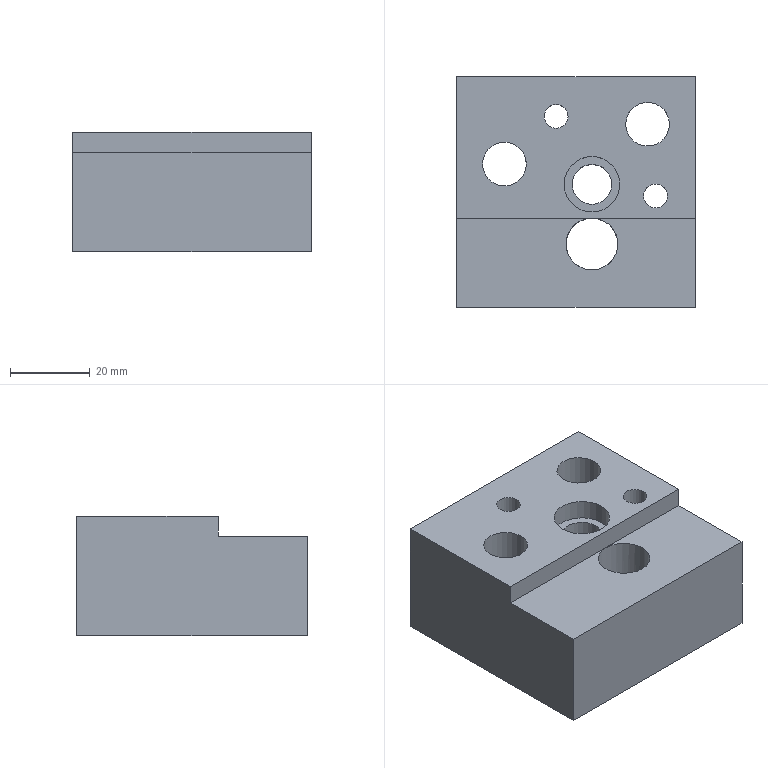Part | NX | features solid 2 | 1 solid | 20 faces | box 60 x 58 x 30 mm | volume 80735 mm3 | plane 11 | cylinder 9 | commonest cylinder face diameters 6 x2 11 x2 17.5 x2 10 x1 13 x1 14 x1
STEP:
#1=CARTESIAN_POINT('',(-695.999,-287.091,74.));
#2=VERTEX_POINT('',#1);
#3=CARTESIAN_POINT('',(-690.999,-287.091,74.));
#4=DIRECTION('',(0.,0.,-1.));
#5=DIRECTION('',(-1.,0.,0.));
#6=AXIS2_PLACEMENT_3D('',#3,#4,#5);
#7=CIRCLE('',#6,5.);
#8=EDGE_CURVE('',#2,#2,#7,.F.);
#9=ORIENTED_EDGE('',*,*,#8,.T.);
#10=EDGE_LOOP('',(#9));
#11=FACE_BOUND('',#10,.T.);
#12=CARTESIAN_POINT('',(-725.,-260.,74.));
#13=VERTEX_POINT('',#12);
#14=CARTESIAN_POINT('',(-665.,-260.,74.));
#15=VERTEX_POINT('',#14);
#16=CARTESIAN_POINT('',(-695.663,-260.,74.));
#17=DIRECTION('',(1.,0.,0.));
#18=VECTOR('',#17,1000.);
#19=LINE('',#16,#18);
#20=EDGE_CURVE('',#13,#15,#19,.T.);
#21=ORIENTED_EDGE('',*,*,#20,.T.);
#22=CARTESIAN_POINT('',(-665.,-318.,74.));
#23=VERTEX_POINT('',#22);
#24=CARTESIAN_POINT('',(-665.,-290.591,74.));
#25=DIRECTION('',(0.,-1.,0.));
#26=VECTOR('',#25,1000.);
#27=LINE('',#24,#26);
#28=EDGE_CURVE('',#15,#23,#27,.T.);
#29=ORIENTED_EDGE('',*,*,#28,.T.);
#30=CARTESIAN_POINT('',(-725.,-318.,74.));
#31=VERTEX_POINT('',#30);
#32=CARTESIAN_POINT('',(-695.663,-318.,74.));
#33=DIRECTION('',(1.,0.,0.));
#34=VECTOR('',#33,1000.);
#35=LINE('',#32,#34);
#36=EDGE_CURVE('',#31,#23,#35,.T.);
#37=ORIENTED_EDGE('',*,*,#36,.F.);
#38=CARTESIAN_POINT('',(-725.,-290.591,74.));
#39=DIRECTION('',(0.,-1.,0.));
#40=VECTOR('',#39,1000.);
#41=LINE('',#38,#40);
#42=EDGE_CURVE('',#13,#31,#41,.T.);
#43=ORIENTED_EDGE('',*,*,#42,.F.);
#44=EDGE_LOOP('',(#21,#29,#37,#43));
#45=FACE_BOUND('',#44,.T.);
#46=CARTESIAN_POINT('',(-668.25,-272.,74.));
#47=VERTEX_POINT('',#46);
#48=CARTESIAN_POINT('',(-677.,-272.,74.));
#49=DIRECTION('',(0.,0.,1.));
#50=DIRECTION('',(1.,0.,0.));
#51=AXIS2_PLACEMENT_3D('',#48,#49,#50);
#52=CIRCLE('',#51,8.75);
#53=EDGE_CURVE('',#47,#47,#52,.T.);
#54=ORIENTED_EDGE('',*,*,#53,.T.);
#55=EDGE_LOOP('',(#54));
#56=FACE_BOUND('',#55,.T.);
#57=CARTESIAN_POINT('',(-704.25,-282.,74.));
#58=VERTEX_POINT('',#57);
#59=CARTESIAN_POINT('',(-713.,-282.,74.));
#60=DIRECTION('',(0.,0.,1.));
#61=DIRECTION('',(1.,0.,0.));
#62=AXIS2_PLACEMENT_3D('',#59,#60,#61);
#63=CIRCLE('',#62,8.75);
#64=EDGE_CURVE('',#58,#58,#63,.T.);
#65=ORIENTED_EDGE('',*,*,#64,.T.);
#66=EDGE_LOOP('',(#65));
#67=FACE_BOUND('',#66,.T.);
#68=CARTESIAN_POINT('',(-697.,-270.,74.));
#69=VERTEX_POINT('',#68);
#70=CARTESIAN_POINT('',(-700.,-270.,74.));
#71=DIRECTION('',(0.,0.,1.));
#72=DIRECTION('',(1.,0.,0.));
#73=AXIS2_PLACEMENT_3D('',#70,#71,#72);
#74=CIRCLE('',#73,3.);
#75=EDGE_CURVE('',#69,#69,#74,.T.);
#76=ORIENTED_EDGE('',*,*,#75,.T.);
#77=EDGE_LOOP('',(#76));
#78=FACE_BOUND('',#77,.T.);
#79=CARTESIAN_POINT('',(-672.,-290.,74.));
#80=VERTEX_POINT('',#79);
#81=CARTESIAN_POINT('',(-675.,-290.,74.));
#82=DIRECTION('',(0.,0.,1.));
#83=DIRECTION('',(1.,0.,0.));
#84=AXIS2_PLACEMENT_3D('',#81,#82,#83);
#85=CIRCLE('',#84,3.);
#86=EDGE_CURVE('',#80,#80,#85,.T.);
#87=ORIENTED_EDGE('',*,*,#86,.T.);
#88=EDGE_LOOP('',(#87));
#89=FACE_BOUND('',#88,.T.);
#90=CARTESIAN_POINT('',(-684.499,-302.091,74.));
#91=VERTEX_POINT('',#90);
#92=CARTESIAN_POINT('',(-690.999,-302.091,74.));
#93=DIRECTION('',(0.,0.,1.));
#94=DIRECTION('',(1.,0.,0.));
#95=AXIS2_PLACEMENT_3D('',#92,#93,#94);
#96=CIRCLE('',#95,6.5);
#97=EDGE_CURVE('',#91,#91,#96,.F.);
#98=ORIENTED_EDGE('',*,*,#97,.F.);
#99=EDGE_LOOP('',(#98));
#100=FACE_BOUND('',#99,.T.);
#101=CARTESIAN_POINT('',(-695.663,-290.591,74.));
#102=DIRECTION('',(0.,0.,-1.));
#103=DIRECTION('',(-1.,0.,0.));
#104=AXIS2_PLACEMENT_3D('',#101,#102,#103);
#105=PLANE('',#104);
#106=ADVANCED_FACE('',(#11,#45,#56,#67,#78,#89,#100),#105,.T.);
#107=CARTESIAN_POINT('',(-665.,-295.591,99.));
#108=VERTEX_POINT('',#107);
#109=CARTESIAN_POINT('',(-665.,-295.591,104.));
#110=VERTEX_POINT('',#109);
#111=CARTESIAN_POINT('',(-665.,-295.591,107.));
#112=DIRECTION('',(0.,0.,1.));
#113=VECTOR('',#112,1000.);
#114=LINE('',#111,#113);
#115=EDGE_CURVE('',#108,#110,#114,.T.);
#116=ORIENTED_EDGE('',*,*,#115,.F.);
#117=CARTESIAN_POINT('',(-665.,-318.,99.));
#118=VERTEX_POINT('',#117);
#119=CARTESIAN_POINT('',(-665.,-302.091,99.));
#120=DIRECTION('',(0.,1.,0.));
#121=VECTOR('',#120,1000.);
#122=LINE('',#119,#121);
#123=EDGE_CURVE('',#108,#118,#122,.F.);
#124=ORIENTED_EDGE('',*,*,#123,.T.);
#125=CARTESIAN_POINT('',(-665.,-318.,0.));
#126=DIRECTION('',(0.,0.,-1.));
#127=VECTOR('',#126,1000.);
#128=LINE('',#125,#127);
#129=EDGE_CURVE('',#118,#23,#128,.T.);
#130=ORIENTED_EDGE('',*,*,#129,.T.);
#131=ORIENTED_EDGE('',*,*,#28,.F.);
#132=CARTESIAN_POINT('',(-665.,-260.,104.));
#133=VERTEX_POINT('',#132);
#134=CARTESIAN_POINT('',(-665.,-260.,0.));
#135=DIRECTION('',(0.,0.,-1.));
#136=VECTOR('',#135,1000.);
#137=LINE('',#134,#136);
#138=EDGE_CURVE('',#133,#15,#137,.T.);
#139=ORIENTED_EDGE('',*,*,#138,.F.);
#140=CARTESIAN_POINT('',(-665.,-302.091,104.));
#141=DIRECTION('',(0.,1.,0.));
#142=VECTOR('',#141,1000.);
#143=LINE('',#140,#142);
#144=EDGE_CURVE('',#133,#110,#143,.F.);
#145=ORIENTED_EDGE('',*,*,#144,.T.);
#146=EDGE_LOOP('',(#116,#124,#130,#131,#139,#145));
#147=FACE_BOUND('',#146,.T.);
#148=CARTESIAN_POINT('',(-665.,0.,0.));
#149=DIRECTION('',(1.,0.,0.));
#150=DIRECTION('',(0.,0.,-1.));
#151=AXIS2_PLACEMENT_3D('',#148,#149,#150);
#152=PLANE('',#151);
#153=ADVANCED_FACE('',(#147),#152,.T.);
#154=CARTESIAN_POINT('',(-725.,-260.,104.));
#155=VERTEX_POINT('',#154);
#156=CARTESIAN_POINT('',(-725.,-260.,0.));
#157=DIRECTION('',(0.,0.,-1.));
#158=VECTOR('',#157,1000.);
#159=LINE('',#156,#158);
#160=EDGE_CURVE('',#155,#13,#159,.T.);
#161=ORIENTED_EDGE('',*,*,#160,.T.);
#162=ORIENTED_EDGE('',*,*,#42,.T.);
#163=CARTESIAN_POINT('',(-725.,-318.,99.));
#164=VERTEX_POINT('',#163);
#165=CARTESIAN_POINT('',(-725.,-318.,0.));
#166=DIRECTION('',(0.,0.,-1.));
#167=VECTOR('',#166,1000.);
#168=LINE('',#165,#167);
#169=EDGE_CURVE('',#164,#31,#168,.T.);
#170=ORIENTED_EDGE('',*,*,#169,.F.);
#171=CARTESIAN_POINT('',(-725.,-295.591,99.));
#172=VERTEX_POINT('',#171);
#173=CARTESIAN_POINT('',(-725.,-302.091,99.));
#174=DIRECTION('',(0.,1.,0.));
#175=VECTOR('',#174,1000.);
#176=LINE('',#173,#175);
#177=EDGE_CURVE('',#172,#164,#176,.F.);
#178=ORIENTED_EDGE('',*,*,#177,.F.);
#179=CARTESIAN_POINT('',(-725.,-295.591,104.));
#180=VERTEX_POINT('',#179);
#181=CARTESIAN_POINT('',(-725.,-295.591,107.));
#182=DIRECTION('',(0.,0.,1.));
#183=VECTOR('',#182,1000.);
#184=LINE('',#181,#183);
#185=EDGE_CURVE('',#172,#180,#184,.T.);
#186=ORIENTED_EDGE('',*,*,#185,.T.);
#187=CARTESIAN_POINT('',(-725.,-302.091,104.));
#188=DIRECTION('',(0.,1.,0.));
#189=VECTOR('',#188,1000.);
#190=LINE('',#187,#189);
#191=EDGE_CURVE('',#155,#180,#190,.F.);
#192=ORIENTED_EDGE('',*,*,#191,.F.);
#193=EDGE_LOOP('',(#161,#162,#170,#178,#186,#192));
#194=FACE_BOUND('',#193,.T.);
#195=CARTESIAN_POINT('',(-725.,0.,0.));
#196=DIRECTION('',(1.,0.,0.));
#197=DIRECTION('',(0.,0.,-1.));
#198=AXIS2_PLACEMENT_3D('',#195,#196,#197);
#199=PLANE('',#198);
#200=ADVANCED_FACE('',(#194),#199,.F.);
#201=CARTESIAN_POINT('',(-672.,-290.,104.));
#202=VERTEX_POINT('',#201);
#203=CARTESIAN_POINT('',(-675.,-290.,104.));
#204=DIRECTION('',(0.,0.,1.));
#205=DIRECTION('',(1.,0.,0.));
#206=AXIS2_PLACEMENT_3D('',#203,#204,#205);
#207=CIRCLE('',#206,3.);
#208=EDGE_CURVE('',#202,#202,#207,.F.);
#209=ORIENTED_EDGE('',*,*,#208,.T.);
#210=EDGE_LOOP('',(#209));
#211=FACE_BOUND('',#210,.T.);
#212=CARTESIAN_POINT('',(-697.,-270.,104.));
#213=VERTEX_POINT('',#212);
#214=CARTESIAN_POINT('',(-700.,-270.,104.));
#215=DIRECTION('',(0.,0.,1.));
#216=DIRECTION('',(1.,0.,0.));
#217=AXIS2_PLACEMENT_3D('',#214,#215,#216);
#218=CIRCLE('',#217,3.);
#219=EDGE_CURVE('',#213,#213,#218,.F.);
#220=ORIENTED_EDGE('',*,*,#219,.T.);
#221=EDGE_LOOP('',(#220));
#222=FACE_BOUND('',#221,.T.);
#223=CARTESIAN_POINT('',(-707.5,-282.,104.));
#224=VERTEX_POINT('',#223);
#225=CARTESIAN_POINT('',(-713.,-282.,104.));
#226=DIRECTION('',(0.,0.,1.));
#227=DIRECTION('',(1.,0.,0.));
#228=AXIS2_PLACEMENT_3D('',#225,#226,#227);
#229=CIRCLE('',#228,5.5);
#230=EDGE_CURVE('',#224,#224,#229,.F.);
#231=ORIENTED_EDGE('',*,*,#230,.T.);
#232=EDGE_LOOP('',(#231));
#233=FACE_BOUND('',#232,.T.);
#234=CARTESIAN_POINT('',(-671.5,-272.,104.));
#235=VERTEX_POINT('',#234);
#236=CARTESIAN_POINT('',(-677.,-272.,104.));
#237=DIRECTION('',(0.,0.,1.));
#238=DIRECTION('',(1.,0.,0.));
#239=AXIS2_PLACEMENT_3D('',#236,#237,#238);
#240=CIRCLE('',#239,5.5);
#241=EDGE_CURVE('',#235,#235,#240,.F.);
#242=ORIENTED_EDGE('',*,*,#241,.T.);
#243=EDGE_LOOP('',(#242));
#244=FACE_BOUND('',#243,.T.);
#245=CARTESIAN_POINT('',(-697.999,-287.091,104.));
#246=VERTEX_POINT('',#245);
#247=CARTESIAN_POINT('',(-690.999,-287.091,104.));
#248=DIRECTION('',(0.,0.,-1.));
#249=DIRECTION('',(-1.,0.,0.));
#250=AXIS2_PLACEMENT_3D('',#247,#248,#249);
#251=CIRCLE('',#250,7.);
#252=EDGE_CURVE('',#246,#246,#251,.F.);
#253=ORIENTED_EDGE('',*,*,#252,.F.);
#254=EDGE_LOOP('',(#253));
#255=FACE_BOUND('',#254,.T.);
#256=ORIENTED_EDGE('',*,*,#144,.F.);
#257=CARTESIAN_POINT('',(-690.999,-260.,104.));
#258=DIRECTION('',(-1.,0.,0.));
#259=VECTOR('',#258,1000.);
#260=LINE('',#257,#259);
#261=EDGE_CURVE('',#155,#133,#260,.F.);
#262=ORIENTED_EDGE('',*,*,#261,.F.);
#263=ORIENTED_EDGE('',*,*,#191,.T.);
#264=CARTESIAN_POINT('',(-686.336,-295.591,104.));
#265=DIRECTION('',(-1.,0.,0.));
#266=VECTOR('',#265,1000.);
#267=LINE('',#264,#266);
#268=EDGE_CURVE('',#180,#110,#267,.F.);
#269=ORIENTED_EDGE('',*,*,#268,.T.);
#270=EDGE_LOOP('',(#256,#262,#263,#269));
#271=FACE_BOUND('',#270,.T.);
#272=CARTESIAN_POINT('',(-690.999,-302.091,104.));
#273=DIRECTION('',(0.,0.,1.));
#274=DIRECTION('',(0.,-1.,0.));
#275=AXIS2_PLACEMENT_3D('',#272,#273,#274);
#276=PLANE('',#275);
#277=ADVANCED_FACE('',(#211,#222,#233,#244,#255,#271),#276,.T.);
#278=ORIENTED_EDGE('',*,*,#261,.T.);
#279=ORIENTED_EDGE('',*,*,#138,.T.);
#280=ORIENTED_EDGE('',*,*,#20,.F.);
#281=ORIENTED_EDGE('',*,*,#160,.F.);
#282=EDGE_LOOP('',(#278,#279,#280,#281));
#283=FACE_BOUND('',#282,.T.);
#284=CARTESIAN_POINT('',(0.,-260.,0.));
#285=DIRECTION('',(0.,1.,0.));
#286=DIRECTION('',(0.,0.,1.));
#287=AXIS2_PLACEMENT_3D('',#284,#285,#286);
#288=PLANE('',#287);
#289=ADVANCED_FACE('',(#283),#288,.T.);
#290=CARTESIAN_POINT('',(-690.999,-295.591,99.));
#291=VERTEX_POINT('',#290);
#292=CARTESIAN_POINT('',(-686.336,-295.591,99.));
#293=DIRECTION('',(-1.,0.,0.));
#294=VECTOR('',#293,1000.);
#295=LINE('',#292,#294);
#296=EDGE_CURVE('',#172,#291,#295,.F.);
#297=ORIENTED_EDGE('',*,*,#296,.F.);
#298=ORIENTED_EDGE('',*,*,#177,.T.);
#299=CARTESIAN_POINT('',(-690.999,-318.,99.));
#300=DIRECTION('',(-1.,0.,0.));
#301=VECTOR('',#300,1000.);
#302=LINE('',#299,#301);
#303=EDGE_CURVE('',#164,#118,#302,.F.);
#304=ORIENTED_EDGE('',*,*,#303,.T.);
#305=ORIENTED_EDGE('',*,*,#123,.F.);
#306=CARTESIAN_POINT('',(-686.336,-295.591,99.));
#307=DIRECTION('',(-1.,0.,0.));
#308=VECTOR('',#307,1000.);
#309=LINE('',#306,#308);
#310=EDGE_CURVE('',#291,#108,#309,.F.);
#311=ORIENTED_EDGE('',*,*,#310,.F.);
#312=CARTESIAN_POINT('',(-690.999,-302.091,99.));
#313=DIRECTION('',(0.,0.,1.));
#314=DIRECTION('',(0.,-1.,0.));
#315=AXIS2_PLACEMENT_3D('',#312,#313,#314);
#316=CIRCLE('',#315,6.5);
#317=EDGE_CURVE('',#291,#291,#316,.T.);
#318=ORIENTED_EDGE('',*,*,#317,.F.);
#319=EDGE_LOOP('',(#297,#298,#304,#305,#311,#318));
#320=FACE_BOUND('',#319,.T.);
#321=CARTESIAN_POINT('',(-690.999,-302.091,99.));
#322=DIRECTION('',(0.,0.,1.));
#323=DIRECTION('',(0.,-1.,0.));
#324=AXIS2_PLACEMENT_3D('',#321,#322,#323);
#325=PLANE('',#324);
#326=ADVANCED_FACE('',(#320),#325,.T.);
#327=ORIENTED_EDGE('',*,*,#115,.T.);
#328=ORIENTED_EDGE('',*,*,#268,.F.);
#329=ORIENTED_EDGE('',*,*,#185,.F.);
#330=ORIENTED_EDGE('',*,*,#296,.T.);
#331=ORIENTED_EDGE('',*,*,#310,.T.);
#332=EDGE_LOOP('',(#327,#328,#329,#330,#331));
#333=FACE_BOUND('',#332,.T.);
#334=CARTESIAN_POINT('',(-686.336,-295.591,107.));
#335=DIRECTION('',(0.,-1.,0.));
#336=DIRECTION('',(1.,0.,0.));
#337=AXIS2_PLACEMENT_3D('',#334,#335,#336);
#338=PLANE('',#337);
#339=ADVANCED_FACE('',(#333),#338,.T.);
#340=ORIENTED_EDGE('',*,*,#129,.F.);
#341=ORIENTED_EDGE('',*,*,#303,.F.);
#342=ORIENTED_EDGE('',*,*,#169,.T.);
#343=ORIENTED_EDGE('',*,*,#36,.T.);
#344=EDGE_LOOP('',(#340,#341,#342,#343));
#345=FACE_BOUND('',#344,.T.);
#346=CARTESIAN_POINT('',(0.,-318.,0.));
#347=DIRECTION('',(0.,1.,0.));
#348=DIRECTION('',(0.,0.,1.));
#349=AXIS2_PLACEMENT_3D('',#346,#347,#348);
#350=PLANE('',#349);
#351=ADVANCED_FACE('',(#345),#350,.F.);
#352=ORIENTED_EDGE('',*,*,#8,.F.);
#353=EDGE_LOOP('',(#352));
#354=FACE_BOUND('',#353,.T.);
#355=CARTESIAN_POINT('',(-685.999,-287.091,99.));
#356=VERTEX_POINT('',#355);
#357=CARTESIAN_POINT('',(-690.999,-287.091,99.));
#358=DIRECTION('',(0.,0.,1.));
#359=DIRECTION('',(1.,0.,0.));
#360=AXIS2_PLACEMENT_3D('',#357,#358,#359);
#361=CIRCLE('',#360,5.);
#362=EDGE_CURVE('',#356,#356,#361,.T.);
#363=ORIENTED_EDGE('',*,*,#362,.T.);
#364=EDGE_LOOP('',(#363));
#365=FACE_BOUND('',#364,.T.);
#366=CARTESIAN_POINT('',(-690.999,-287.091,104.));
#367=DIRECTION('',(0.,0.,-1.));
#368=DIRECTION('',(-1.,0.,0.));
#369=AXIS2_PLACEMENT_3D('',#366,#367,#368);
#370=CYLINDRICAL_SURFACE('',#369,5.);
#371=ADVANCED_FACE('',(#354,#365),#370,.F.);
#372=CARTESIAN_POINT('',(-697.999,-287.091,99.));
#373=VERTEX_POINT('',#372);
#374=CARTESIAN_POINT('',(-690.999,-287.091,99.));
#375=DIRECTION('',(0.,0.,-1.));
#376=DIRECTION('',(-1.,0.,0.));
#377=AXIS2_PLACEMENT_3D('',#374,#375,#376);
#378=CIRCLE('',#377,7.);
#379=EDGE_CURVE('',#373,#373,#378,.F.);
#380=ORIENTED_EDGE('',*,*,#379,.T.);
#381=EDGE_LOOP('',(#380));
#382=FACE_BOUND('',#381,.T.);
#383=ORIENTED_EDGE('',*,*,#362,.F.);
#384=EDGE_LOOP('',(#383));
#385=FACE_BOUND('',#384,.T.);
#386=CARTESIAN_POINT('',(-690.999,-287.091,99.));
#387=DIRECTION('',(0.,0.,1.));
#388=DIRECTION('',(1.,0.,0.));
#389=AXIS2_PLACEMENT_3D('',#386,#387,#388);
#390=PLANE('',#389);
#391=ADVANCED_FACE('',(#382,#385),#390,.T.);
#392=ORIENTED_EDGE('',*,*,#379,.F.);
#393=EDGE_LOOP('',(#392));
#394=FACE_BOUND('',#393,.T.);
#395=ORIENTED_EDGE('',*,*,#252,.T.);
#396=EDGE_LOOP('',(#395));
#397=FACE_BOUND('',#396,.T.);
#398=CARTESIAN_POINT('',(-690.999,-287.091,99.));
#399=DIRECTION('',(0.,0.,1.));
#400=DIRECTION('',(1.,0.,0.));
#401=AXIS2_PLACEMENT_3D('',#398,#399,#400);
#402=CYLINDRICAL_SURFACE('',#401,7.);
#403=ADVANCED_FACE('',(#394,#397),#402,.F.);
#404=CARTESIAN_POINT('',(-682.5,-272.,86.));
#405=VERTEX_POINT('',#404);
#406=CARTESIAN_POINT('',(-677.,-272.,86.));
#407=DIRECTION('',(0.,0.,-1.));
#408=DIRECTION('',(-1.,0.,0.));
#409=AXIS2_PLACEMENT_3D('',#406,#407,#408);
#410=CIRCLE('',#409,5.5);
#411=EDGE_CURVE('',#405,#405,#410,.F.);
#412=ORIENTED_EDGE('',*,*,#411,.F.);
#413=EDGE_LOOP('',(#412));
#414=FACE_BOUND('',#413,.T.);
#415=ORIENTED_EDGE('',*,*,#241,.F.);
#416=EDGE_LOOP('',(#415));
#417=FACE_BOUND('',#416,.T.);
#418=CARTESIAN_POINT('',(-677.,-272.,124.));
#419=DIRECTION('',(0.,0.,1.));
#420=DIRECTION('',(1.,0.,0.));
#421=AXIS2_PLACEMENT_3D('',#418,#419,#420);
#422=CYLINDRICAL_SURFACE('',#421,5.5);
#423=ADVANCED_FACE('',(#414,#417),#422,.F.);
#424=ORIENTED_EDGE('',*,*,#411,.T.);
#425=EDGE_LOOP('',(#424));
#426=FACE_BOUND('',#425,.T.);
#427=CARTESIAN_POINT('',(-685.75,-272.,86.));
#428=VERTEX_POINT('',#427);
#429=CARTESIAN_POINT('',(-677.,-272.,86.));
#430=DIRECTION('',(0.,0.,-1.));
#431=DIRECTION('',(-1.,0.,0.));
#432=AXIS2_PLACEMENT_3D('',#429,#430,#431);
#433=CIRCLE('',#432,8.75);
#434=EDGE_CURVE('',#428,#428,#433,.F.);
#435=ORIENTED_EDGE('',*,*,#434,.F.);
#436=EDGE_LOOP('',(#435));
#437=FACE_BOUND('',#436,.T.);
#438=CARTESIAN_POINT('',(-677.,-272.,86.));
#439=DIRECTION('',(0.,0.,1.));
#440=DIRECTION('',(1.,0.,0.));
#441=AXIS2_PLACEMENT_3D('',#438,#439,#440);
#442=PLANE('',#441);
#443=ADVANCED_FACE('',(#426,#437),#442,.F.);
#444=ORIENTED_EDGE('',*,*,#434,.T.);
#445=EDGE_LOOP('',(#444));
#446=FACE_BOUND('',#445,.T.);
#447=ORIENTED_EDGE('',*,*,#53,.F.);
#448=EDGE_LOOP('',(#447));
#449=FACE_BOUND('',#448,.T.);
#450=CARTESIAN_POINT('',(-677.,-272.,74.));
#451=DIRECTION('',(0.,0.,1.));
#452=DIRECTION('',(1.,0.,0.));
#453=AXIS2_PLACEMENT_3D('',#450,#451,#452);
#454=CYLINDRICAL_SURFACE('',#453,8.75);
#455=ADVANCED_FACE('',(#446,#449),#454,.F.);
#456=CARTESIAN_POINT('',(-718.5,-282.,86.));
#457=VERTEX_POINT('',#456);
#458=CARTESIAN_POINT('',(-713.,-282.,86.));
#459=DIRECTION('',(0.,0.,-1.));
#460=DIRECTION('',(-1.,0.,0.));
#461=AXIS2_PLACEMENT_3D('',#458,#459,#460);
#462=CIRCLE('',#461,5.5);
#463=EDGE_CURVE('',#457,#457,#462,.F.);
#464=ORIENTED_EDGE('',*,*,#463,.F.);
#465=EDGE_LOOP('',(#464));
#466=FACE_BOUND('',#465,.T.);
#467=ORIENTED_EDGE('',*,*,#230,.F.);
#468=EDGE_LOOP('',(#467));
#469=FACE_BOUND('',#468,.T.);
#470=CARTESIAN_POINT('',(-713.,-282.,124.));
#471=DIRECTION('',(0.,0.,1.));
#472=DIRECTION('',(1.,0.,0.));
#473=AXIS2_PLACEMENT_3D('',#470,#471,#472);
#474=CYLINDRICAL_SURFACE('',#473,5.5);
#475=ADVANCED_FACE('',(#466,#469),#474,.F.);
#476=ORIENTED_EDGE('',*,*,#463,.T.);
#477=EDGE_LOOP('',(#476));
#478=FACE_BOUND('',#477,.T.);
#479=CARTESIAN_POINT('',(-721.75,-282.,86.));
#480=VERTEX_POINT('',#479);
#481=CARTESIAN_POINT('',(-713.,-282.,86.));
#482=DIRECTION('',(0.,0.,-1.));
#483=DIRECTION('',(-1.,0.,0.));
#484=AXIS2_PLACEMENT_3D('',#481,#482,#483);
#485=CIRCLE('',#484,8.75);
#486=EDGE_CURVE('',#480,#480,#485,.F.);
#487=ORIENTED_EDGE('',*,*,#486,.F.);
#488=EDGE_LOOP('',(#487));
#489=FACE_BOUND('',#488,.T.);
#490=CARTESIAN_POINT('',(-713.,-272.,86.));
#491=DIRECTION('',(0.,0.,1.));
#492=DIRECTION('',(1.,0.,0.));
#493=AXIS2_PLACEMENT_3D('',#490,#491,#492);
#494=PLANE('',#493);
#495=ADVANCED_FACE('',(#478,#489),#494,.F.);
#496=ORIENTED_EDGE('',*,*,#486,.T.);
#497=EDGE_LOOP('',(#496));
#498=FACE_BOUND('',#497,.T.);
#499=ORIENTED_EDGE('',*,*,#64,.F.);
#500=EDGE_LOOP('',(#499));
#501=FACE_BOUND('',#500,.T.);
#502=CARTESIAN_POINT('',(-713.,-282.,74.));
#503=DIRECTION('',(0.,0.,1.));
#504=DIRECTION('',(1.,0.,0.));
#505=AXIS2_PLACEMENT_3D('',#502,#503,#504);
#506=CYLINDRICAL_SURFACE('',#505,8.75);
#507=ADVANCED_FACE('',(#498,#501),#506,.F.);
#508=ORIENTED_EDGE('',*,*,#75,.F.);
#509=EDGE_LOOP('',(#508));
#510=FACE_BOUND('',#509,.T.);
#511=ORIENTED_EDGE('',*,*,#219,.F.);
#512=EDGE_LOOP('',(#511));
#513=FACE_BOUND('',#512,.T.);
#514=CARTESIAN_POINT('',(-700.,-270.,74.));
#515=DIRECTION('',(0.,0.,1.));
#516=DIRECTION('',(1.,0.,0.));
#517=AXIS2_PLACEMENT_3D('',#514,#515,#516);
#518=CYLINDRICAL_SURFACE('',#517,3.);
#519=ADVANCED_FACE('',(#510,#513),#518,.F.);
#520=ORIENTED_EDGE('',*,*,#86,.F.);
#521=EDGE_LOOP('',(#520));
#522=FACE_BOUND('',#521,.T.);
#523=ORIENTED_EDGE('',*,*,#208,.F.);
#524=EDGE_LOOP('',(#523));
#525=FACE_BOUND('',#524,.T.);
#526=CARTESIAN_POINT('',(-675.,-290.,74.));
#527=DIRECTION('',(0.,0.,1.));
#528=DIRECTION('',(1.,0.,0.));
#529=AXIS2_PLACEMENT_3D('',#526,#527,#528);
#530=CYLINDRICAL_SURFACE('',#529,3.);
#531=ADVANCED_FACE('',(#522,#525),#530,.F.);
#532=ORIENTED_EDGE('',*,*,#97,.T.);
#533=EDGE_LOOP('',(#532));
#534=FACE_BOUND('',#533,.T.);
#535=ORIENTED_EDGE('',*,*,#317,.T.);
#536=EDGE_LOOP('',(#535));
#537=FACE_BOUND('',#536,.T.);
#538=CARTESIAN_POINT('',(-690.999,-302.091,104.));
#539=DIRECTION('',(0.,0.,-1.));
#540=DIRECTION('',(0.,1.,0.));
#541=AXIS2_PLACEMENT_3D('',#538,#539,#540);
#542=CYLINDRICAL_SURFACE('',#541,6.5);
#543=ADVANCED_FACE('',(#534,#537),#542,.F.);
#544=CLOSED_SHELL('',(#106,#153,#200,#277,#289,#326,#339,#351,#371,#391,#403,#423,#443,#455,#475,#495,#507,#519,#531,#543));
#545=MANIFOLD_SOLID_BREP('',#544);
#546=(LENGTH_UNIT()NAMED_UNIT(*)SI_UNIT(.MILLI.,.METRE.));
#547=UNCERTAINTY_MEASURE_WITH_UNIT(LENGTH_MEASURE(0.00001),#546,'','');
#548=(NAMED_UNIT(*)PLANE_ANGLE_UNIT()SI_UNIT($,.RADIAN.));
#549=(NAMED_UNIT(*)SI_UNIT($,.STERADIAN.)SOLID_ANGLE_UNIT());
#550=(GEOMETRIC_REPRESENTATION_CONTEXT(3)GLOBAL_UNCERTAINTY_ASSIGNED_CONTEXT((#547))GLOBAL_UNIT_ASSIGNED_CONTEXT((#546,#548,#549))REPRESENTATION_CONTEXT('',''));
#551=ADVANCED_BREP_SHAPE_REPRESENTATION('',(#545),#550);